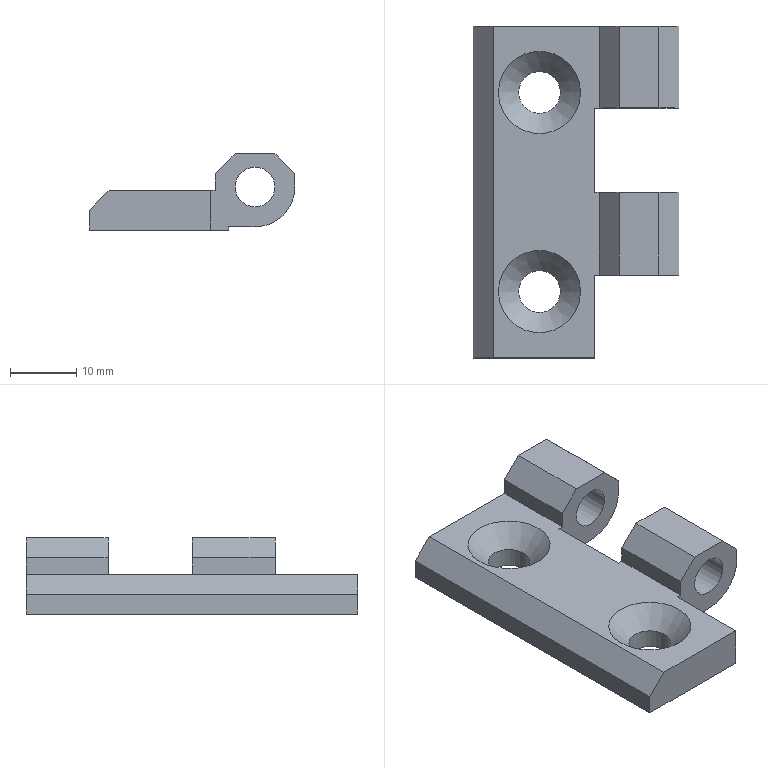Part | STEP file | C_HHSZ50_pr | 1 solid | 33 faces | box 31 x 50 x 11.5 mm | volume 6935 mm3 | plane 25 | cylinder 6 | cone 2 | commonest cylinder face diameters 6 x2 6.3 x2 12 x2
STEP:
#1=CARTESIAN_POINT('',(-11.85,15.,0.));
#2=VERTEX_POINT('',#1);
#3=CARTESIAN_POINT('',(-15.,15.,0.));
#4=DIRECTION('',(0.,0.,1.));
#5=DIRECTION('',(1.,0.,0.));
#6=AXIS2_PLACEMENT_3D('',#3,#4,#5);
#7=CIRCLE('',#6,3.15);
#8=EDGE_CURVE('',#2,#2,#7,.T.);
#9=ORIENTED_EDGE('',*,*,#8,.T.);
#10=EDGE_LOOP('',(#9));
#11=FACE_BOUND('',#10,.T.);
#12=CARTESIAN_POINT('',(-4.,12.65,0.));
#13=VERTEX_POINT('',#12);
#14=CARTESIAN_POINT('',(-6.7,12.65,0.));
#15=VERTEX_POINT('',#14);
#16=CARTESIAN_POINT('',(6.7,12.65,0.));
#17=DIRECTION('',(-1.,0.,0.));
#18=VECTOR('',#17,1000.);
#19=LINE('',#16,#18);
#20=EDGE_CURVE('',#13,#15,#19,.T.);
#21=ORIENTED_EDGE('',*,*,#20,.T.);
#22=CARTESIAN_POINT('',(-6.7,-0.05,0.));
#23=VERTEX_POINT('',#22);
#24=CARTESIAN_POINT('',(-6.7,12.65,0.));
#25=DIRECTION('',(0.,-1.,0.));
#26=VECTOR('',#25,1000.);
#27=LINE('',#24,#26);
#28=EDGE_CURVE('',#15,#23,#27,.T.);
#29=ORIENTED_EDGE('',*,*,#28,.T.);
#30=CARTESIAN_POINT('',(-4.,-0.05,0.));
#31=VERTEX_POINT('',#30);
#32=CARTESIAN_POINT('',(-6.7,-0.05,0.));
#33=DIRECTION('',(1.,0.,0.));
#34=VECTOR('',#33,1000.);
#35=LINE('',#32,#34);
#36=EDGE_CURVE('',#23,#31,#35,.T.);
#37=ORIENTED_EDGE('',*,*,#36,.T.);
#38=CARTESIAN_POINT('',(-4.,-12.55,0.));
#39=VERTEX_POINT('',#38);
#40=CARTESIAN_POINT('',(-4.,25.,0.));
#41=DIRECTION('',(0.,-1.,0.));
#42=VECTOR('',#41,1000.);
#43=LINE('',#40,#42);
#44=EDGE_CURVE('',#31,#39,#43,.T.);
#45=ORIENTED_EDGE('',*,*,#44,.T.);
#46=CARTESIAN_POINT('',(-6.7,-12.55,0.));
#47=VERTEX_POINT('',#46);
#48=CARTESIAN_POINT('',(6.7,-12.55,0.));
#49=DIRECTION('',(-1.,0.,0.));
#50=VECTOR('',#49,1000.);
#51=LINE('',#48,#50);
#52=EDGE_CURVE('',#39,#47,#51,.T.);
#53=ORIENTED_EDGE('',*,*,#52,.T.);
#54=CARTESIAN_POINT('',(-6.7,-25.,0.));
#55=VERTEX_POINT('',#54);
#56=CARTESIAN_POINT('',(-6.7,-12.55,0.));
#57=DIRECTION('',(0.,-1.,0.));
#58=VECTOR('',#57,1000.);
#59=LINE('',#56,#58);
#60=EDGE_CURVE('',#47,#55,#59,.T.);
#61=ORIENTED_EDGE('',*,*,#60,.T.);
#62=CARTESIAN_POINT('',(-25.,-25.,0.));
#63=VERTEX_POINT('',#62);
#64=CARTESIAN_POINT('',(-4.,-25.,0.));
#65=DIRECTION('',(-1.,0.,0.));
#66=VECTOR('',#65,1000.);
#67=LINE('',#64,#66);
#68=EDGE_CURVE('',#55,#63,#67,.T.);
#69=ORIENTED_EDGE('',*,*,#68,.T.);
#70=CARTESIAN_POINT('',(-25.,25.,0.));
#71=VERTEX_POINT('',#70);
#72=CARTESIAN_POINT('',(-25.,25.,0.));
#73=DIRECTION('',(0.,-1.,0.));
#74=VECTOR('',#73,1000.);
#75=LINE('',#72,#74);
#76=EDGE_CURVE('',#71,#63,#75,.T.);
#77=ORIENTED_EDGE('',*,*,#76,.F.);
#78=CARTESIAN_POINT('',(-4.,25.,0.));
#79=VERTEX_POINT('',#78);
#80=CARTESIAN_POINT('',(-4.,25.,0.));
#81=DIRECTION('',(-1.,0.,0.));
#82=VECTOR('',#81,1000.);
#83=LINE('',#80,#82);
#84=EDGE_CURVE('',#79,#71,#83,.T.);
#85=ORIENTED_EDGE('',*,*,#84,.F.);
#86=CARTESIAN_POINT('',(-4.,25.,0.));
#87=DIRECTION('',(0.,-1.,0.));
#88=VECTOR('',#87,1000.);
#89=LINE('',#86,#88);
#90=EDGE_CURVE('',#79,#13,#89,.T.);
#91=ORIENTED_EDGE('',*,*,#90,.T.);
#92=EDGE_LOOP('',(#21,#29,#37,#45,#53,#61,#69,#77,#85,#91));
#93=FACE_OUTER_BOUND('',#92,.T.);
#94=CARTESIAN_POINT('',(-11.85,-15.,0.));
#95=VERTEX_POINT('',#94);
#96=CARTESIAN_POINT('',(-15.,-15.,0.));
#97=DIRECTION('',(0.,0.,1.));
#98=DIRECTION('',(1.,0.,0.));
#99=AXIS2_PLACEMENT_3D('',#96,#97,#98);
#100=CIRCLE('',#99,3.15);
#101=EDGE_CURVE('',#95,#95,#100,.T.);
#102=ORIENTED_EDGE('',*,*,#101,.T.);
#103=EDGE_LOOP('',(#102));
#104=FACE_BOUND('',#103,.T.);
#105=CARTESIAN_POINT('',(-4.,25.,0.));
#106=DIRECTION('',(0.,0.,1.));
#107=DIRECTION('',(1.,0.,0.));
#108=AXIS2_PLACEMENT_3D('',#105,#106,#107);
#109=PLANE('',#108);
#110=ADVANCED_FACE('',(#11,#93,#104),#109,.F.);
#111=CARTESIAN_POINT('',(-8.8,15.,6.));
#112=VERTEX_POINT('',#111);
#113=CARTESIAN_POINT('',(-15.,15.,6.));
#114=DIRECTION('',(0.,0.,1.));
#115=DIRECTION('',(1.,0.,0.));
#116=AXIS2_PLACEMENT_3D('',#113,#114,#115);
#117=CIRCLE('',#116,6.2);
#118=EDGE_CURVE('',#112,#112,#117,.T.);
#119=ORIENTED_EDGE('',*,*,#118,.F.);
#120=EDGE_LOOP('',(#119));
#121=FACE_BOUND('',#120,.T.);
#122=CARTESIAN_POINT('',(-6.,12.65,6.));
#123=VERTEX_POINT('',#122);
#124=CARTESIAN_POINT('',(-6.7,12.65,6.));
#125=VERTEX_POINT('',#124);
#126=CARTESIAN_POINT('',(-22.,12.65,6.));
#127=DIRECTION('',(-1.,0.,0.));
#128=VECTOR('',#127,1000.);
#129=LINE('',#126,#128);
#130=EDGE_CURVE('',#123,#125,#129,.T.);
#131=ORIENTED_EDGE('',*,*,#130,.F.);
#132=CARTESIAN_POINT('',(-6.,25.,6.));
#133=VERTEX_POINT('',#132);
#134=CARTESIAN_POINT('',(-6.,25.,6.));
#135=DIRECTION('',(0.,-1.,0.));
#136=VECTOR('',#135,1000.);
#137=LINE('',#134,#136);
#138=EDGE_CURVE('',#133,#123,#137,.T.);
#139=ORIENTED_EDGE('',*,*,#138,.F.);
#140=CARTESIAN_POINT('',(-22.,25.,6.));
#141=VERTEX_POINT('',#140);
#142=CARTESIAN_POINT('',(-22.,25.,6.));
#143=DIRECTION('',(1.,0.,0.));
#144=VECTOR('',#143,1000.);
#145=LINE('',#142,#144);
#146=EDGE_CURVE('',#141,#133,#145,.T.);
#147=ORIENTED_EDGE('',*,*,#146,.F.);
#148=CARTESIAN_POINT('',(-22.,-25.,6.));
#149=VERTEX_POINT('',#148);
#150=CARTESIAN_POINT('',(-22.,25.,6.));
#151=DIRECTION('',(0.,-1.,0.));
#152=VECTOR('',#151,1000.);
#153=LINE('',#150,#152);
#154=EDGE_CURVE('',#141,#149,#153,.T.);
#155=ORIENTED_EDGE('',*,*,#154,.T.);
#156=CARTESIAN_POINT('',(-6.7,-25.,6.));
#157=VERTEX_POINT('',#156);
#158=CARTESIAN_POINT('',(-22.,-25.,6.));
#159=DIRECTION('',(1.,0.,0.));
#160=VECTOR('',#159,1000.);
#161=LINE('',#158,#160);
#162=EDGE_CURVE('',#149,#157,#161,.T.);
#163=ORIENTED_EDGE('',*,*,#162,.T.);
#164=CARTESIAN_POINT('',(-6.7,-12.55,6.));
#165=VERTEX_POINT('',#164);
#166=CARTESIAN_POINT('',(-6.7,25.,6.));
#167=DIRECTION('',(0.,-1.,0.));
#168=VECTOR('',#167,1000.);
#169=LINE('',#166,#168);
#170=EDGE_CURVE('',#165,#157,#169,.T.);
#171=ORIENTED_EDGE('',*,*,#170,.F.);
#172=CARTESIAN_POINT('',(-6.,-12.55,6.));
#173=VERTEX_POINT('',#172);
#174=CARTESIAN_POINT('',(-22.,-12.55,6.));
#175=DIRECTION('',(-1.,0.,0.));
#176=VECTOR('',#175,1000.);
#177=LINE('',#174,#176);
#178=EDGE_CURVE('',#173,#165,#177,.T.);
#179=ORIENTED_EDGE('',*,*,#178,.F.);
#180=CARTESIAN_POINT('',(-6.,-0.05,6.));
#181=VERTEX_POINT('',#180);
#182=CARTESIAN_POINT('',(-6.,25.,6.));
#183=DIRECTION('',(0.,-1.,0.));
#184=VECTOR('',#183,1000.);
#185=LINE('',#182,#184);
#186=EDGE_CURVE('',#181,#173,#185,.T.);
#187=ORIENTED_EDGE('',*,*,#186,.F.);
#188=CARTESIAN_POINT('',(-6.7,-0.05,6.));
#189=VERTEX_POINT('',#188);
#190=CARTESIAN_POINT('',(-22.,-0.05,6.));
#191=DIRECTION('',(1.,0.,0.));
#192=VECTOR('',#191,1000.);
#193=LINE('',#190,#192);
#194=EDGE_CURVE('',#189,#181,#193,.T.);
#195=ORIENTED_EDGE('',*,*,#194,.F.);
#196=CARTESIAN_POINT('',(-6.7,25.,6.));
#197=DIRECTION('',(0.,-1.,0.));
#198=VECTOR('',#197,1000.);
#199=LINE('',#196,#198);
#200=EDGE_CURVE('',#125,#189,#199,.T.);
#201=ORIENTED_EDGE('',*,*,#200,.F.);
#202=EDGE_LOOP('',(#131,#139,#147,#155,#163,#171,#179,#187,#195,#201));
#203=FACE_OUTER_BOUND('',#202,.T.);
#204=CARTESIAN_POINT('',(-8.8,-15.,6.));
#205=VERTEX_POINT('',#204);
#206=CARTESIAN_POINT('',(-15.,-15.,6.));
#207=DIRECTION('',(0.,0.,1.));
#208=DIRECTION('',(1.,0.,0.));
#209=AXIS2_PLACEMENT_3D('',#206,#207,#208);
#210=CIRCLE('',#209,6.2);
#211=EDGE_CURVE('',#205,#205,#210,.T.);
#212=ORIENTED_EDGE('',*,*,#211,.F.);
#213=EDGE_LOOP('',(#212));
#214=FACE_BOUND('',#213,.T.);
#215=CARTESIAN_POINT('',(-22.,25.,6.));
#216=DIRECTION('',(0.,0.,-1.));
#217=DIRECTION('',(-1.,0.,0.));
#218=AXIS2_PLACEMENT_3D('',#215,#216,#217);
#219=PLANE('',#218);
#220=ADVANCED_FACE('',(#121,#203,#214),#219,.F.);
#221=CARTESIAN_POINT('',(-6.,12.65,8.5));
#222=VERTEX_POINT('',#221);
#223=CARTESIAN_POINT('',(-6.,12.65,6.));
#224=DIRECTION('',(0.,0.,-1.));
#225=VECTOR('',#224,1000.);
#226=LINE('',#223,#225);
#227=EDGE_CURVE('',#222,#123,#226,.T.);
#228=ORIENTED_EDGE('',*,*,#227,.F.);
#229=CARTESIAN_POINT('',(-6.,25.,8.5));
#230=VERTEX_POINT('',#229);
#231=CARTESIAN_POINT('',(-6.,25.,8.5));
#232=DIRECTION('',(0.,-1.,0.));
#233=VECTOR('',#232,1000.);
#234=LINE('',#231,#233);
#235=EDGE_CURVE('',#230,#222,#234,.T.);
#236=ORIENTED_EDGE('',*,*,#235,.F.);
#237=CARTESIAN_POINT('',(-6.,25.,6.));
#238=DIRECTION('',(0.,0.,1.));
#239=VECTOR('',#238,1000.);
#240=LINE('',#237,#239);
#241=EDGE_CURVE('',#133,#230,#240,.T.);
#242=ORIENTED_EDGE('',*,*,#241,.F.);
#243=ORIENTED_EDGE('',*,*,#138,.T.);
#244=EDGE_LOOP('',(#228,#236,#242,#243));
#245=FACE_OUTER_BOUND('',#244,.T.);
#246=CARTESIAN_POINT('',(-6.,25.,6.));
#247=DIRECTION('',(1.,0.,0.));
#248=DIRECTION('',(0.,0.,-1.));
#249=AXIS2_PLACEMENT_3D('',#246,#247,#248);
#250=PLANE('',#249);
#251=ADVANCED_FACE('',(#245),#250,.F.);
#252=CARTESIAN_POINT('',(-6.,-0.05,8.5));
#253=VERTEX_POINT('',#252);
#254=CARTESIAN_POINT('',(-6.,-0.05,6.));
#255=DIRECTION('',(0.,0.,1.));
#256=VECTOR('',#255,1000.);
#257=LINE('',#254,#256);
#258=EDGE_CURVE('',#181,#253,#257,.T.);
#259=ORIENTED_EDGE('',*,*,#258,.F.);
#260=ORIENTED_EDGE('',*,*,#186,.T.);
#261=CARTESIAN_POINT('',(-6.,-12.55,8.5));
#262=VERTEX_POINT('',#261);
#263=CARTESIAN_POINT('',(-6.,-12.55,6.));
#264=DIRECTION('',(0.,0.,-1.));
#265=VECTOR('',#264,1000.);
#266=LINE('',#263,#265);
#267=EDGE_CURVE('',#262,#173,#266,.T.);
#268=ORIENTED_EDGE('',*,*,#267,.F.);
#269=CARTESIAN_POINT('',(-6.,25.,8.5));
#270=DIRECTION('',(0.,-1.,0.));
#271=VECTOR('',#270,1000.);
#272=LINE('',#269,#271);
#273=EDGE_CURVE('',#253,#262,#272,.T.);
#274=ORIENTED_EDGE('',*,*,#273,.F.);
#275=EDGE_LOOP('',(#259,#260,#268,#274));
#276=FACE_OUTER_BOUND('',#275,.T.);
#277=CARTESIAN_POINT('',(-6.,25.,6.));
#278=DIRECTION('',(1.,0.,0.));
#279=DIRECTION('',(0.,0.,-1.));
#280=AXIS2_PLACEMENT_3D('',#277,#278,#279);
#281=PLANE('',#280);
#282=ADVANCED_FACE('',(#276),#281,.F.);
#283=CARTESIAN_POINT('',(-3.,12.65,11.5));
#284=VERTEX_POINT('',#283);
#285=CARTESIAN_POINT('',(-6.,12.65,8.5));
#286=DIRECTION('',(-0.7071,0.,-0.7071));
#287=VECTOR('',#286,1000.);
#288=LINE('',#285,#287);
#289=EDGE_CURVE('',#284,#222,#288,.T.);
#290=ORIENTED_EDGE('',*,*,#289,.F.);
#291=CARTESIAN_POINT('',(-3.,25.,11.5));
#292=VERTEX_POINT('',#291);
#293=CARTESIAN_POINT('',(-3.,25.,11.5));
#294=DIRECTION('',(0.,-1.,0.));
#295=VECTOR('',#294,1000.);
#296=LINE('',#293,#295);
#297=EDGE_CURVE('',#292,#284,#296,.T.);
#298=ORIENTED_EDGE('',*,*,#297,.F.);
#299=CARTESIAN_POINT('',(-6.,25.,8.5));
#300=DIRECTION('',(0.7071,0.,0.7071));
#301=VECTOR('',#300,1000.);
#302=LINE('',#299,#301);
#303=EDGE_CURVE('',#230,#292,#302,.T.);
#304=ORIENTED_EDGE('',*,*,#303,.F.);
#305=ORIENTED_EDGE('',*,*,#235,.T.);
#306=EDGE_LOOP('',(#290,#298,#304,#305));
#307=FACE_OUTER_BOUND('',#306,.T.);
#308=CARTESIAN_POINT('',(-6.,25.,8.5));
#309=DIRECTION('',(0.7071,0.,-0.7071));
#310=DIRECTION('',(-0.7071,0.,-0.7071));
#311=AXIS2_PLACEMENT_3D('',#308,#309,#310);
#312=PLANE('',#311);
#313=ADVANCED_FACE('',(#307),#312,.F.);
#314=CARTESIAN_POINT('',(-3.,-0.05,11.5));
#315=VERTEX_POINT('',#314);
#316=CARTESIAN_POINT('',(-6.,-0.05,8.5));
#317=DIRECTION('',(0.7071,0.,0.7071));
#318=VECTOR('',#317,1000.);
#319=LINE('',#316,#318);
#320=EDGE_CURVE('',#253,#315,#319,.T.);
#321=ORIENTED_EDGE('',*,*,#320,.F.);
#322=ORIENTED_EDGE('',*,*,#273,.T.);
#323=CARTESIAN_POINT('',(-3.,-12.55,11.5));
#324=VERTEX_POINT('',#323);
#325=CARTESIAN_POINT('',(-6.,-12.55,8.5));
#326=DIRECTION('',(-0.7071,0.,-0.7071));
#327=VECTOR('',#326,1000.);
#328=LINE('',#325,#327);
#329=EDGE_CURVE('',#324,#262,#328,.T.);
#330=ORIENTED_EDGE('',*,*,#329,.F.);
#331=CARTESIAN_POINT('',(-3.,25.,11.5));
#332=DIRECTION('',(0.,-1.,0.));
#333=VECTOR('',#332,1000.);
#334=LINE('',#331,#333);
#335=EDGE_CURVE('',#315,#324,#334,.T.);
#336=ORIENTED_EDGE('',*,*,#335,.F.);
#337=EDGE_LOOP('',(#321,#322,#330,#336));
#338=FACE_OUTER_BOUND('',#337,.T.);
#339=CARTESIAN_POINT('',(-6.,25.,8.5));
#340=DIRECTION('',(0.7071,0.,-0.7071));
#341=DIRECTION('',(-0.7071,0.,-0.7071));
#342=AXIS2_PLACEMENT_3D('',#339,#340,#341);
#343=PLANE('',#342);
#344=ADVANCED_FACE('',(#338),#343,.F.);
#345=CARTESIAN_POINT('',(3.,12.65,11.5));
#346=VERTEX_POINT('',#345);
#347=CARTESIAN_POINT('',(-3.,12.65,11.5));
#348=DIRECTION('',(-1.,0.,0.));
#349=VECTOR('',#348,1000.);
#350=LINE('',#347,#349);
#351=EDGE_CURVE('',#346,#284,#350,.T.);
#352=ORIENTED_EDGE('',*,*,#351,.F.);
#353=CARTESIAN_POINT('',(3.,25.,11.5));
#354=VERTEX_POINT('',#353);
#355=CARTESIAN_POINT('',(3.,25.,11.5));
#356=DIRECTION('',(0.,-1.,0.));
#357=VECTOR('',#356,1000.);
#358=LINE('',#355,#357);
#359=EDGE_CURVE('',#354,#346,#358,.T.);
#360=ORIENTED_EDGE('',*,*,#359,.F.);
#361=CARTESIAN_POINT('',(-3.,25.,11.5));
#362=DIRECTION('',(1.,0.,0.));
#363=VECTOR('',#362,1000.);
#364=LINE('',#361,#363);
#365=EDGE_CURVE('',#292,#354,#364,.T.);
#366=ORIENTED_EDGE('',*,*,#365,.F.);
#367=ORIENTED_EDGE('',*,*,#297,.T.);
#368=EDGE_LOOP('',(#352,#360,#366,#367));
#369=FACE_OUTER_BOUND('',#368,.T.);
#370=CARTESIAN_POINT('',(-3.,25.,11.5));
#371=DIRECTION('',(0.,0.,-1.));
#372=DIRECTION('',(-1.,0.,0.));
#373=AXIS2_PLACEMENT_3D('',#370,#371,#372);
#374=PLANE('',#373);
#375=ADVANCED_FACE('',(#369),#374,.F.);
#376=CARTESIAN_POINT('',(3.,-0.05,11.5));
#377=VERTEX_POINT('',#376);
#378=CARTESIAN_POINT('',(-3.,-0.05,11.5));
#379=DIRECTION('',(1.,0.,0.));
#380=VECTOR('',#379,1000.);
#381=LINE('',#378,#380);
#382=EDGE_CURVE('',#315,#377,#381,.T.);
#383=ORIENTED_EDGE('',*,*,#382,.F.);
#384=ORIENTED_EDGE('',*,*,#335,.T.);
#385=CARTESIAN_POINT('',(3.,-12.55,11.5));
#386=VERTEX_POINT('',#385);
#387=CARTESIAN_POINT('',(-3.,-12.55,11.5));
#388=DIRECTION('',(-1.,0.,0.));
#389=VECTOR('',#388,1000.);
#390=LINE('',#387,#389);
#391=EDGE_CURVE('',#386,#324,#390,.T.);
#392=ORIENTED_EDGE('',*,*,#391,.F.);
#393=CARTESIAN_POINT('',(3.,25.,11.5));
#394=DIRECTION('',(0.,-1.,0.));
#395=VECTOR('',#394,1000.);
#396=LINE('',#393,#395);
#397=EDGE_CURVE('',#377,#386,#396,.T.);
#398=ORIENTED_EDGE('',*,*,#397,.F.);
#399=EDGE_LOOP('',(#383,#384,#392,#398));
#400=FACE_OUTER_BOUND('',#399,.T.);
#401=CARTESIAN_POINT('',(-3.,25.,11.5));
#402=DIRECTION('',(0.,0.,-1.));
#403=DIRECTION('',(-1.,0.,0.));
#404=AXIS2_PLACEMENT_3D('',#401,#402,#403);
#405=PLANE('',#404);
#406=ADVANCED_FACE('',(#400),#405,.F.);
#407=CARTESIAN_POINT('',(6.,12.65,8.5));
#408=VERTEX_POINT('',#407);
#409=CARTESIAN_POINT('',(3.,12.65,11.5));
#410=DIRECTION('',(-0.7071,0.,0.7071));
#411=VECTOR('',#410,1000.);
#412=LINE('',#409,#411);
#413=EDGE_CURVE('',#408,#346,#412,.T.);
#414=ORIENTED_EDGE('',*,*,#413,.F.);
#415=CARTESIAN_POINT('',(6.,25.,8.5));
#416=VERTEX_POINT('',#415);
#417=CARTESIAN_POINT('',(6.,25.,8.5));
#418=DIRECTION('',(0.,-1.,0.));
#419=VECTOR('',#418,1000.);
#420=LINE('',#417,#419);
#421=EDGE_CURVE('',#416,#408,#420,.T.);
#422=ORIENTED_EDGE('',*,*,#421,.F.);
#423=CARTESIAN_POINT('',(3.,25.,11.5));
#424=DIRECTION('',(0.7071,0.,-0.7071));
#425=VECTOR('',#424,1000.);
#426=LINE('',#423,#425);
#427=EDGE_CURVE('',#354,#416,#426,.T.);
#428=ORIENTED_EDGE('',*,*,#427,.F.);
#429=ORIENTED_EDGE('',*,*,#359,.T.);
#430=EDGE_LOOP('',(#414,#422,#428,#429));
#431=FACE_OUTER_BOUND('',#430,.T.);
#432=CARTESIAN_POINT('',(3.,25.,11.5));
#433=DIRECTION('',(-0.7071,0.,-0.7071));
#434=DIRECTION('',(-0.7071,0.,0.7071));
#435=AXIS2_PLACEMENT_3D('',#432,#433,#434);
#436=PLANE('',#435);
#437=ADVANCED_FACE('',(#431),#436,.F.);
#438=CARTESIAN_POINT('',(6.,-0.05,8.5));
#439=VERTEX_POINT('',#438);
#440=CARTESIAN_POINT('',(3.,-0.05,11.5));
#441=DIRECTION('',(0.7071,0.,-0.7071));
#442=VECTOR('',#441,1000.);
#443=LINE('',#440,#442);
#444=EDGE_CURVE('',#377,#439,#443,.T.);
#445=ORIENTED_EDGE('',*,*,#444,.F.);
#446=ORIENTED_EDGE('',*,*,#397,.T.);
#447=CARTESIAN_POINT('',(6.,-12.55,8.5));
#448=VERTEX_POINT('',#447);
#449=CARTESIAN_POINT('',(3.,-12.55,11.5));
#450=DIRECTION('',(-0.7071,0.,0.7071));
#451=VECTOR('',#450,1000.);
#452=LINE('',#449,#451);
#453=EDGE_CURVE('',#448,#386,#452,.T.);
#454=ORIENTED_EDGE('',*,*,#453,.F.);
#455=CARTESIAN_POINT('',(6.,25.,8.5));
#456=DIRECTION('',(0.,-1.,0.));
#457=VECTOR('',#456,1000.);
#458=LINE('',#455,#457);
#459=EDGE_CURVE('',#439,#448,#458,.T.);
#460=ORIENTED_EDGE('',*,*,#459,.F.);
#461=EDGE_LOOP('',(#445,#446,#454,#460));
#462=FACE_OUTER_BOUND('',#461,.T.);
#463=CARTESIAN_POINT('',(3.,25.,11.5));
#464=DIRECTION('',(-0.7071,0.,-0.7071));
#465=DIRECTION('',(-0.7071,0.,0.7071));
#466=AXIS2_PLACEMENT_3D('',#463,#464,#465);
#467=PLANE('',#466);
#468=ADVANCED_FACE('',(#462),#467,.F.);
#469=CARTESIAN_POINT('',(6.,12.65,6.5));
#470=VERTEX_POINT('',#469);
#471=CARTESIAN_POINT('',(6.,12.65,8.5));
#472=DIRECTION('',(0.,0.,1.));
#473=VECTOR('',#472,1000.);
#474=LINE('',#471,#473);
#475=EDGE_CURVE('',#470,#408,#474,.T.);
#476=ORIENTED_EDGE('',*,*,#475,.F.);
#477=CARTESIAN_POINT('',(6.,25.,6.5));
#478=VERTEX_POINT('',#477);
#479=CARTESIAN_POINT('',(6.,25.,6.5));
#480=DIRECTION('',(0.,-1.,0.));
#481=VECTOR('',#480,1000.);
#482=LINE('',#479,#481);
#483=EDGE_CURVE('',#478,#470,#482,.T.);
#484=ORIENTED_EDGE('',*,*,#483,.F.);
#485=CARTESIAN_POINT('',(6.,25.,8.5));
#486=DIRECTION('',(0.,0.,-1.));
#487=VECTOR('',#486,1000.);
#488=LINE('',#485,#487);
#489=EDGE_CURVE('',#416,#478,#488,.T.);
#490=ORIENTED_EDGE('',*,*,#489,.F.);
#491=ORIENTED_EDGE('',*,*,#421,.T.);
#492=EDGE_LOOP('',(#476,#484,#490,#491));
#493=FACE_OUTER_BOUND('',#492,.T.);
#494=CARTESIAN_POINT('',(6.,25.,8.5));
#495=DIRECTION('',(-1.,0.,0.));
#496=DIRECTION('',(0.,0.,1.));
#497=AXIS2_PLACEMENT_3D('',#494,#495,#496);
#498=PLANE('',#497);
#499=ADVANCED_FACE('',(#493),#498,.F.);
#500=CARTESIAN_POINT('',(6.,-0.05,6.5));
#501=VERTEX_POINT('',#500);
#502=CARTESIAN_POINT('',(6.,-0.05,8.5));
#503=DIRECTION('',(0.,0.,-1.));
#504=VECTOR('',#503,1000.);
#505=LINE('',#502,#504);
#506=EDGE_CURVE('',#439,#501,#505,.T.);
#507=ORIENTED_EDGE('',*,*,#506,.F.);
#508=ORIENTED_EDGE('',*,*,#459,.T.);
#509=CARTESIAN_POINT('',(6.,-12.55,6.5));
#510=VERTEX_POINT('',#509);
#511=CARTESIAN_POINT('',(6.,-12.55,8.5));
#512=DIRECTION('',(0.,0.,1.));
#513=VECTOR('',#512,1000.);
#514=LINE('',#511,#513);
#515=EDGE_CURVE('',#510,#448,#514,.T.);
#516=ORIENTED_EDGE('',*,*,#515,.F.);
#517=CARTESIAN_POINT('',(6.,25.,6.5));
#518=DIRECTION('',(0.,-1.,0.));
#519=VECTOR('',#518,1000.);
#520=LINE('',#517,#519);
#521=EDGE_CURVE('',#501,#510,#520,.T.);
#522=ORIENTED_EDGE('',*,*,#521,.F.);
#523=EDGE_LOOP('',(#507,#508,#516,#522));
#524=FACE_OUTER_BOUND('',#523,.T.);
#525=CARTESIAN_POINT('',(6.,25.,8.5));
#526=DIRECTION('',(-1.,0.,0.));
#527=DIRECTION('',(0.,0.,1.));
#528=AXIS2_PLACEMENT_3D('',#525,#526,#527);
#529=PLANE('',#528);
#530=ADVANCED_FACE('',(#524),#529,.F.);
#531=CARTESIAN_POINT('',(0.,12.65,0.5));
#532=VERTEX_POINT('',#531);
#533=CARTESIAN_POINT('',(0.,12.65,6.5));
#534=DIRECTION('',(0.,-1.,0.));
#535=DIRECTION('',(0.,0.,-1.));
#536=AXIS2_PLACEMENT_3D('',#533,#534,#535);
#537=CIRCLE('',#536,6.);
#538=EDGE_CURVE('',#532,#470,#537,.T.);
#539=ORIENTED_EDGE('',*,*,#538,.F.);
#540=CARTESIAN_POINT('',(0.,25.,0.5));
#541=VERTEX_POINT('',#540);
#542=CARTESIAN_POINT('',(0.,25.,0.5));
#543=DIRECTION('',(0.,-1.,0.));
#544=VECTOR('',#543,1000.);
#545=LINE('',#542,#544);
#546=EDGE_CURVE('',#541,#532,#545,.T.);
#547=ORIENTED_EDGE('',*,*,#546,.F.);
#548=CARTESIAN_POINT('',(0.,25.,6.5));
#549=DIRECTION('',(0.,1.,0.));
#550=DIRECTION('',(0.,0.,1.));
#551=AXIS2_PLACEMENT_3D('',#548,#549,#550);
#552=CIRCLE('',#551,6.);
#553=EDGE_CURVE('',#478,#541,#552,.T.);
#554=ORIENTED_EDGE('',*,*,#553,.F.);
#555=ORIENTED_EDGE('',*,*,#483,.T.);
#556=EDGE_LOOP('',(#539,#547,#554,#555));
#557=FACE_OUTER_BOUND('',#556,.T.);
#558=CARTESIAN_POINT('',(0.,25.,6.5));
#559=DIRECTION('',(0.,-1.,0.));
#560=DIRECTION('',(0.,0.,-1.));
#561=AXIS2_PLACEMENT_3D('',#558,#559,#560);
#562=CYLINDRICAL_SURFACE('',#561,6.);
#563=ADVANCED_FACE('',(#557),#562,.T.);
#564=CARTESIAN_POINT('',(0.,-0.05,0.5));
#565=VERTEX_POINT('',#564);
#566=CARTESIAN_POINT('',(0.,-0.05,6.5));
#567=DIRECTION('',(0.,1.,0.));
#568=DIRECTION('',(0.,0.,1.));
#569=AXIS2_PLACEMENT_3D('',#566,#567,#568);
#570=CIRCLE('',#569,6.);
#571=EDGE_CURVE('',#501,#565,#570,.T.);
#572=ORIENTED_EDGE('',*,*,#571,.F.);
#573=ORIENTED_EDGE('',*,*,#521,.T.);
#574=CARTESIAN_POINT('',(0.,-12.55,0.5));
#575=VERTEX_POINT('',#574);
#576=CARTESIAN_POINT('',(0.,-12.55,6.5));
#577=DIRECTION('',(0.,-1.,0.));
#578=DIRECTION('',(0.,0.,-1.));
#579=AXIS2_PLACEMENT_3D('',#576,#577,#578);
#580=CIRCLE('',#579,6.);
#581=EDGE_CURVE('',#575,#510,#580,.T.);
#582=ORIENTED_EDGE('',*,*,#581,.F.);
#583=CARTESIAN_POINT('',(0.,25.,0.5));
#584=DIRECTION('',(0.,-1.,0.));
#585=VECTOR('',#584,1000.);
#586=LINE('',#583,#585);
#587=EDGE_CURVE('',#565,#575,#586,.T.);
#588=ORIENTED_EDGE('',*,*,#587,.F.);
#589=EDGE_LOOP('',(#572,#573,#582,#588));
#590=FACE_OUTER_BOUND('',#589,.T.);
#591=CARTESIAN_POINT('',(0.,25.,6.5));
#592=DIRECTION('',(0.,-1.,0.));
#593=DIRECTION('',(0.,0.,-1.));
#594=AXIS2_PLACEMENT_3D('',#591,#592,#593);
#595=CYLINDRICAL_SURFACE('',#594,6.);
#596=ADVANCED_FACE('',(#590),#595,.T.);
#597=CARTESIAN_POINT('',(-4.,12.65,0.5));
#598=VERTEX_POINT('',#597);
#599=CARTESIAN_POINT('',(0.,12.65,0.5));
#600=DIRECTION('',(1.,0.,0.));
#601=VECTOR('',#600,1000.);
#602=LINE('',#599,#601);
#603=EDGE_CURVE('',#598,#532,#602,.T.);
#604=ORIENTED_EDGE('',*,*,#603,.F.);
#605=CARTESIAN_POINT('',(-4.,25.,0.5));
#606=VERTEX_POINT('',#605);
#607=CARTESIAN_POINT('',(-4.,25.,0.5));
#608=DIRECTION('',(0.,-1.,0.));
#609=VECTOR('',#608,1000.);
#610=LINE('',#607,#609);
#611=EDGE_CURVE('',#606,#598,#610,.T.);
#612=ORIENTED_EDGE('',*,*,#611,.F.);
#613=CARTESIAN_POINT('',(0.,25.,0.5));
#614=DIRECTION('',(-1.,0.,0.));
#615=VECTOR('',#614,1000.);
#616=LINE('',#613,#615);
#617=EDGE_CURVE('',#541,#606,#616,.T.);
#618=ORIENTED_EDGE('',*,*,#617,.F.);
#619=ORIENTED_EDGE('',*,*,#546,.T.);
#620=EDGE_LOOP('',(#604,#612,#618,#619));
#621=FACE_OUTER_BOUND('',#620,.T.);
#622=CARTESIAN_POINT('',(0.,25.,0.5));
#623=DIRECTION('',(0.,0.,1.));
#624=DIRECTION('',(1.,0.,0.));
#625=AXIS2_PLACEMENT_3D('',#622,#623,#624);
#626=PLANE('',#625);
#627=ADVANCED_FACE('',(#621),#626,.F.);
#628=CARTESIAN_POINT('',(-4.,-0.05,0.5));
#629=VERTEX_POINT('',#628);
#630=CARTESIAN_POINT('',(0.,-0.05,0.5));
#631=DIRECTION('',(-1.,0.,0.));
#632=VECTOR('',#631,1000.);
#633=LINE('',#630,#632);
#634=EDGE_CURVE('',#565,#629,#633,.T.);
#635=ORIENTED_EDGE('',*,*,#634,.F.);
#636=ORIENTED_EDGE('',*,*,#587,.T.);
#637=CARTESIAN_POINT('',(-4.,-12.55,0.5));
#638=VERTEX_POINT('',#637);
#639=CARTESIAN_POINT('',(0.,-12.55,0.5));
#640=DIRECTION('',(1.,0.,0.));
#641=VECTOR('',#640,1000.);
#642=LINE('',#639,#641);
#643=EDGE_CURVE('',#638,#575,#642,.T.);
#644=ORIENTED_EDGE('',*,*,#643,.F.);
#645=CARTESIAN_POINT('',(-4.,25.,0.5));
#646=DIRECTION('',(0.,-1.,0.));
#647=VECTOR('',#646,1000.);
#648=LINE('',#645,#647);
#649=EDGE_CURVE('',#629,#638,#648,.T.);
#650=ORIENTED_EDGE('',*,*,#649,.F.);
#651=EDGE_LOOP('',(#635,#636,#644,#650));
#652=FACE_OUTER_BOUND('',#651,.T.);
#653=CARTESIAN_POINT('',(0.,25.,0.5));
#654=DIRECTION('',(0.,0.,1.));
#655=DIRECTION('',(1.,0.,0.));
#656=AXIS2_PLACEMENT_3D('',#653,#654,#655);
#657=PLANE('',#656);
#658=ADVANCED_FACE('',(#652),#657,.F.);
#659=CARTESIAN_POINT('',(-4.,12.65,0.5));
#660=DIRECTION('',(0.,0.,1.));
#661=VECTOR('',#660,1000.);
#662=LINE('',#659,#661);
#663=EDGE_CURVE('',#13,#598,#662,.T.);
#664=ORIENTED_EDGE('',*,*,#663,.F.);
#665=ORIENTED_EDGE('',*,*,#90,.F.);
#666=CARTESIAN_POINT('',(-4.,25.,0.5));
#667=DIRECTION('',(0.,0.,-1.));
#668=VECTOR('',#667,1000.);
#669=LINE('',#666,#668);
#670=EDGE_CURVE('',#606,#79,#669,.T.);
#671=ORIENTED_EDGE('',*,*,#670,.F.);
#672=ORIENTED_EDGE('',*,*,#611,.T.);
#673=EDGE_LOOP('',(#664,#665,#671,#672));
#674=FACE_OUTER_BOUND('',#673,.T.);
#675=CARTESIAN_POINT('',(-4.,25.,0.5));
#676=DIRECTION('',(-1.,0.,0.));
#677=DIRECTION('',(0.,0.,1.));
#678=AXIS2_PLACEMENT_3D('',#675,#676,#677);
#679=PLANE('',#678);
#680=ADVANCED_FACE('',(#674),#679,.F.);
#681=CARTESIAN_POINT('',(-4.,-0.05,0.5));
#682=DIRECTION('',(0.,0.,-1.));
#683=VECTOR('',#682,1000.);
#684=LINE('',#681,#683);
#685=EDGE_CURVE('',#629,#31,#684,.T.);
#686=ORIENTED_EDGE('',*,*,#685,.F.);
#687=ORIENTED_EDGE('',*,*,#649,.T.);
#688=CARTESIAN_POINT('',(-4.,-12.55,0.5));
#689=DIRECTION('',(0.,0.,1.));
#690=VECTOR('',#689,1000.);
#691=LINE('',#688,#690);
#692=EDGE_CURVE('',#39,#638,#691,.T.);
#693=ORIENTED_EDGE('',*,*,#692,.F.);
#694=ORIENTED_EDGE('',*,*,#44,.F.);
#695=EDGE_LOOP('',(#686,#687,#693,#694));
#696=FACE_OUTER_BOUND('',#695,.T.);
#697=CARTESIAN_POINT('',(-4.,25.,0.5));
#698=DIRECTION('',(-1.,0.,0.));
#699=DIRECTION('',(0.,0.,1.));
#700=AXIS2_PLACEMENT_3D('',#697,#698,#699);
#701=PLANE('',#700);
#702=ADVANCED_FACE('',(#696),#701,.F.);
#703=CARTESIAN_POINT('',(0.,25.,9.5));
#704=VERTEX_POINT('',#703);
#705=CARTESIAN_POINT('',(0.,25.,6.5));
#706=DIRECTION('',(0.,1.,0.));
#707=DIRECTION('',(0.,0.,1.));
#708=AXIS2_PLACEMENT_3D('',#705,#706,#707);
#709=CIRCLE('',#708,3.);
#710=EDGE_CURVE('',#704,#704,#709,.T.);
#711=ORIENTED_EDGE('',*,*,#710,.T.);
#712=EDGE_LOOP('',(#711));
#713=FACE_OUTER_BOUND('',#712,.T.);
#714=CARTESIAN_POINT('',(0.,12.65,3.5));
#715=VERTEX_POINT('',#714);
#716=CARTESIAN_POINT('',(0.,12.65,6.5));
#717=DIRECTION('',(0.,-1.,0.));
#718=DIRECTION('',(0.,0.,-1.));
#719=AXIS2_PLACEMENT_3D('',#716,#717,#718);
#720=CIRCLE('',#719,3.);
#721=EDGE_CURVE('',#715,#715,#720,.T.);
#722=ORIENTED_EDGE('',*,*,#721,.T.);
#723=EDGE_LOOP('',(#722));
#724=FACE_OUTER_BOUND('',#723,.T.);
#725=CARTESIAN_POINT('',(0.,-25.,6.5));
#726=DIRECTION('',(0.,1.,0.));
#727=DIRECTION('',(0.,0.,1.));
#728=AXIS2_PLACEMENT_3D('',#725,#726,#727);
#729=CYLINDRICAL_SURFACE('',#728,3.);
#730=ADVANCED_FACE('',(#713,#724),#729,.F.);
#731=CARTESIAN_POINT('',(0.,-12.55,3.5));
#732=VERTEX_POINT('',#731);
#733=CARTESIAN_POINT('',(0.,-12.55,6.5));
#734=DIRECTION('',(0.,-1.,0.));
#735=DIRECTION('',(0.,0.,-1.));
#736=AXIS2_PLACEMENT_3D('',#733,#734,#735);
#737=CIRCLE('',#736,3.);
#738=EDGE_CURVE('',#732,#732,#737,.T.);
#739=ORIENTED_EDGE('',*,*,#738,.T.);
#740=EDGE_LOOP('',(#739));
#741=FACE_OUTER_BOUND('',#740,.T.);
#742=CARTESIAN_POINT('',(0.,-0.05,9.5));
#743=VERTEX_POINT('',#742);
#744=CARTESIAN_POINT('',(0.,-0.05,6.5));
#745=DIRECTION('',(0.,1.,0.));
#746=DIRECTION('',(0.,0.,1.));
#747=AXIS2_PLACEMENT_3D('',#744,#745,#746);
#748=CIRCLE('',#747,3.);
#749=EDGE_CURVE('',#743,#743,#748,.T.);
#750=ORIENTED_EDGE('',*,*,#749,.T.);
#751=EDGE_LOOP('',(#750));
#752=FACE_OUTER_BOUND('',#751,.T.);
#753=CARTESIAN_POINT('',(0.,-25.,6.5));
#754=DIRECTION('',(0.,1.,0.));
#755=DIRECTION('',(0.,0.,1.));
#756=AXIS2_PLACEMENT_3D('',#753,#754,#755);
#757=CYLINDRICAL_SURFACE('',#756,3.);
#758=ADVANCED_FACE('',(#741,#752),#757,.F.);
#759=CARTESIAN_POINT('',(-6.7,-25.,12.));
#760=DIRECTION('',(0.,0.,-1.));
#761=VECTOR('',#760,1000.);
#762=LINE('',#759,#761);
#763=EDGE_CURVE('',#157,#55,#762,.T.);
#764=ORIENTED_EDGE('',*,*,#763,.F.);
#765=ORIENTED_EDGE('',*,*,#162,.F.);
#766=CARTESIAN_POINT('',(-25.,-25.,3.));
#767=VERTEX_POINT('',#766);
#768=CARTESIAN_POINT('',(-25.,-25.,3.));
#769=DIRECTION('',(0.7071,0.,0.7071));
#770=VECTOR('',#769,1000.);
#771=LINE('',#768,#770);
#772=EDGE_CURVE('',#767,#149,#771,.T.);
#773=ORIENTED_EDGE('',*,*,#772,.F.);
#774=CARTESIAN_POINT('',(-25.,-25.,0.));
#775=DIRECTION('',(0.,0.,1.));
#776=VECTOR('',#775,1000.);
#777=LINE('',#774,#776);
#778=EDGE_CURVE('',#63,#767,#777,.T.);
#779=ORIENTED_EDGE('',*,*,#778,.F.);
#780=ORIENTED_EDGE('',*,*,#68,.F.);
#781=EDGE_LOOP('',(#764,#765,#773,#779,#780));
#782=FACE_OUTER_BOUND('',#781,.T.);
#783=CARTESIAN_POINT('',(0.,-25.,6.5));
#784=DIRECTION('',(0.,1.,0.));
#785=DIRECTION('',(0.,0.,1.));
#786=AXIS2_PLACEMENT_3D('',#783,#784,#785);
#787=PLANE('',#786);
#788=ADVANCED_FACE('',(#782),#787,.F.);
#789=ORIENTED_EDGE('',*,*,#84,.T.);
#790=CARTESIAN_POINT('',(-25.,25.,3.));
#791=VERTEX_POINT('',#790);
#792=CARTESIAN_POINT('',(-25.,25.,0.));
#793=DIRECTION('',(0.,0.,1.));
#794=VECTOR('',#793,1000.);
#795=LINE('',#792,#794);
#796=EDGE_CURVE('',#71,#791,#795,.T.);
#797=ORIENTED_EDGE('',*,*,#796,.T.);
#798=CARTESIAN_POINT('',(-25.,25.,3.));
#799=DIRECTION('',(0.7071,0.,0.7071));
#800=VECTOR('',#799,1000.);
#801=LINE('',#798,#800);
#802=EDGE_CURVE('',#791,#141,#801,.T.);
#803=ORIENTED_EDGE('',*,*,#802,.T.);
#804=ORIENTED_EDGE('',*,*,#146,.T.);
#805=ORIENTED_EDGE('',*,*,#241,.T.);
#806=ORIENTED_EDGE('',*,*,#303,.T.);
#807=ORIENTED_EDGE('',*,*,#365,.T.);
#808=ORIENTED_EDGE('',*,*,#427,.T.);
#809=ORIENTED_EDGE('',*,*,#489,.T.);
#810=ORIENTED_EDGE('',*,*,#553,.T.);
#811=ORIENTED_EDGE('',*,*,#617,.T.);
#812=ORIENTED_EDGE('',*,*,#670,.T.);
#813=EDGE_LOOP('',(#789,#797,#803,#804,#805,#806,#807,#808,#809,#810,#811,#812));
#814=FACE_OUTER_BOUND('',#813,.T.);
#815=ORIENTED_EDGE('',*,*,#710,.F.);
#816=EDGE_LOOP('',(#815));
#817=FACE_BOUND('',#816,.T.);
#818=CARTESIAN_POINT('',(0.,25.,6.5));
#819=DIRECTION('',(0.,1.,0.));
#820=DIRECTION('',(0.,0.,1.));
#821=AXIS2_PLACEMENT_3D('',#818,#819,#820);
#822=PLANE('',#821);
#823=ADVANCED_FACE('',(#814,#817),#822,.T.);
#824=ORIENTED_EDGE('',*,*,#76,.T.);
#825=ORIENTED_EDGE('',*,*,#778,.T.);
#826=CARTESIAN_POINT('',(-25.,25.,3.));
#827=DIRECTION('',(0.,-1.,0.));
#828=VECTOR('',#827,1000.);
#829=LINE('',#826,#828);
#830=EDGE_CURVE('',#791,#767,#829,.T.);
#831=ORIENTED_EDGE('',*,*,#830,.F.);
#832=ORIENTED_EDGE('',*,*,#796,.F.);
#833=EDGE_LOOP('',(#824,#825,#831,#832));
#834=FACE_OUTER_BOUND('',#833,.T.);
#835=CARTESIAN_POINT('',(-25.,25.,0.));
#836=DIRECTION('',(1.,0.,0.));
#837=DIRECTION('',(0.,0.,-1.));
#838=AXIS2_PLACEMENT_3D('',#835,#836,#837);
#839=PLANE('',#838);
#840=ADVANCED_FACE('',(#834),#839,.F.);
#841=ORIENTED_EDGE('',*,*,#830,.T.);
#842=ORIENTED_EDGE('',*,*,#772,.T.);
#843=ORIENTED_EDGE('',*,*,#154,.F.);
#844=ORIENTED_EDGE('',*,*,#802,.F.);
#845=EDGE_LOOP('',(#841,#842,#843,#844));
#846=FACE_OUTER_BOUND('',#845,.T.);
#847=CARTESIAN_POINT('',(-25.,25.,3.));
#848=DIRECTION('',(0.7071,0.,-0.7071));
#849=DIRECTION('',(-0.7071,0.,-0.7071));
#850=AXIS2_PLACEMENT_3D('',#847,#848,#849);
#851=PLANE('',#850);
#852=ADVANCED_FACE('',(#846),#851,.F.);
#853=ORIENTED_EDGE('',*,*,#170,.T.);
#854=ORIENTED_EDGE('',*,*,#763,.T.);
#855=ORIENTED_EDGE('',*,*,#60,.F.);
#856=CARTESIAN_POINT('',(-6.7,-12.55,12.));
#857=DIRECTION('',(0.,0.,-1.));
#858=VECTOR('',#857,1000.);
#859=LINE('',#856,#858);
#860=EDGE_CURVE('',#165,#47,#859,.T.);
#861=ORIENTED_EDGE('',*,*,#860,.F.);
#862=EDGE_LOOP('',(#853,#854,#855,#861));
#863=FACE_OUTER_BOUND('',#862,.T.);
#864=CARTESIAN_POINT('',(-6.7,-12.55,12.));
#865=DIRECTION('',(1.,0.,0.));
#866=DIRECTION('',(0.,0.,-1.));
#867=AXIS2_PLACEMENT_3D('',#864,#865,#866);
#868=PLANE('',#867);
#869=ADVANCED_FACE('',(#863),#868,.T.);
#870=ORIENTED_EDGE('',*,*,#738,.F.);
#871=EDGE_LOOP('',(#870));
#872=FACE_BOUND('',#871,.T.);
#873=ORIENTED_EDGE('',*,*,#178,.T.);
#874=ORIENTED_EDGE('',*,*,#860,.T.);
#875=ORIENTED_EDGE('',*,*,#52,.F.);
#876=ORIENTED_EDGE('',*,*,#692,.T.);
#877=ORIENTED_EDGE('',*,*,#643,.T.);
#878=ORIENTED_EDGE('',*,*,#581,.T.);
#879=ORIENTED_EDGE('',*,*,#515,.T.);
#880=ORIENTED_EDGE('',*,*,#453,.T.);
#881=ORIENTED_EDGE('',*,*,#391,.T.);
#882=ORIENTED_EDGE('',*,*,#329,.T.);
#883=ORIENTED_EDGE('',*,*,#267,.T.);
#884=EDGE_LOOP('',(#873,#874,#875,#876,#877,#878,#879,#880,#881,#882,#883));
#885=FACE_OUTER_BOUND('',#884,.T.);
#886=CARTESIAN_POINT('',(6.7,-12.55,12.));
#887=DIRECTION('',(0.,-1.,0.));
#888=DIRECTION('',(0.,0.,-1.));
#889=AXIS2_PLACEMENT_3D('',#886,#887,#888);
#890=PLANE('',#889);
#891=ADVANCED_FACE('',(#872,#885),#890,.T.);
#892=ORIENTED_EDGE('',*,*,#200,.T.);
#893=CARTESIAN_POINT('',(-6.7,-0.05,12.));
#894=DIRECTION('',(0.,0.,-1.));
#895=VECTOR('',#894,1000.);
#896=LINE('',#893,#895);
#897=EDGE_CURVE('',#189,#23,#896,.T.);
#898=ORIENTED_EDGE('',*,*,#897,.T.);
#899=ORIENTED_EDGE('',*,*,#28,.F.);
#900=CARTESIAN_POINT('',(-6.7,12.65,12.));
#901=DIRECTION('',(0.,0.,-1.));
#902=VECTOR('',#901,1000.);
#903=LINE('',#900,#902);
#904=EDGE_CURVE('',#125,#15,#903,.T.);
#905=ORIENTED_EDGE('',*,*,#904,.F.);
#906=EDGE_LOOP('',(#892,#898,#899,#905));
#907=FACE_OUTER_BOUND('',#906,.T.);
#908=CARTESIAN_POINT('',(-6.7,12.65,12.));
#909=DIRECTION('',(1.,0.,0.));
#910=DIRECTION('',(0.,0.,-1.));
#911=AXIS2_PLACEMENT_3D('',#908,#909,#910);
#912=PLANE('',#911);
#913=ADVANCED_FACE('',(#907),#912,.T.);
#914=ORIENTED_EDGE('',*,*,#721,.F.);
#915=EDGE_LOOP('',(#914));
#916=FACE_BOUND('',#915,.T.);
#917=ORIENTED_EDGE('',*,*,#130,.T.);
#918=ORIENTED_EDGE('',*,*,#904,.T.);
#919=ORIENTED_EDGE('',*,*,#20,.F.);
#920=ORIENTED_EDGE('',*,*,#663,.T.);
#921=ORIENTED_EDGE('',*,*,#603,.T.);
#922=ORIENTED_EDGE('',*,*,#538,.T.);
#923=ORIENTED_EDGE('',*,*,#475,.T.);
#924=ORIENTED_EDGE('',*,*,#413,.T.);
#925=ORIENTED_EDGE('',*,*,#351,.T.);
#926=ORIENTED_EDGE('',*,*,#289,.T.);
#927=ORIENTED_EDGE('',*,*,#227,.T.);
#928=EDGE_LOOP('',(#917,#918,#919,#920,#921,#922,#923,#924,#925,#926,#927));
#929=FACE_OUTER_BOUND('',#928,.T.);
#930=CARTESIAN_POINT('',(6.7,12.65,12.));
#931=DIRECTION('',(0.,-1.,0.));
#932=DIRECTION('',(0.,0.,-1.));
#933=AXIS2_PLACEMENT_3D('',#930,#931,#932);
#934=PLANE('',#933);
#935=ADVANCED_FACE('',(#916,#929),#934,.T.);
#936=ORIENTED_EDGE('',*,*,#749,.F.);
#937=EDGE_LOOP('',(#936));
#938=FACE_BOUND('',#937,.T.);
#939=ORIENTED_EDGE('',*,*,#194,.T.);
#940=ORIENTED_EDGE('',*,*,#258,.T.);
#941=ORIENTED_EDGE('',*,*,#320,.T.);
#942=ORIENTED_EDGE('',*,*,#382,.T.);
#943=ORIENTED_EDGE('',*,*,#444,.T.);
#944=ORIENTED_EDGE('',*,*,#506,.T.);
#945=ORIENTED_EDGE('',*,*,#571,.T.);
#946=ORIENTED_EDGE('',*,*,#634,.T.);
#947=ORIENTED_EDGE('',*,*,#685,.T.);
#948=ORIENTED_EDGE('',*,*,#36,.F.);
#949=ORIENTED_EDGE('',*,*,#897,.F.);
#950=EDGE_LOOP('',(#939,#940,#941,#942,#943,#944,#945,#946,#947,#948,#949));
#951=FACE_OUTER_BOUND('',#950,.T.);
#952=CARTESIAN_POINT('',(-6.7,-0.05,12.));
#953=DIRECTION('',(0.,1.,0.));
#954=DIRECTION('',(0.,0.,1.));
#955=AXIS2_PLACEMENT_3D('',#952,#953,#954);
#956=PLANE('',#955);
#957=ADVANCED_FACE('',(#938,#951),#956,.T.);
#958=ORIENTED_EDGE('',*,*,#118,.T.);
#959=EDGE_LOOP('',(#958));
#960=FACE_OUTER_BOUND('',#959,.T.);
#961=CARTESIAN_POINT('',(-11.85,15.,2.9));
#962=VERTEX_POINT('',#961);
#963=CARTESIAN_POINT('',(-15.,15.,2.9));
#964=DIRECTION('',(0.,0.,1.));
#965=DIRECTION('',(1.,0.,0.));
#966=AXIS2_PLACEMENT_3D('',#963,#964,#965);
#967=CIRCLE('',#966,3.15);
#968=EDGE_CURVE('',#962,#962,#967,.T.);
#969=ORIENTED_EDGE('',*,*,#968,.F.);
#970=EDGE_LOOP('',(#969));
#971=FACE_BOUND('',#970,.T.);
#972=CARTESIAN_POINT('',(-15.,15.,2.9));
#973=DIRECTION('',(0.,0.,1.));
#974=DIRECTION('',(1.,0.,0.));
#975=AXIS2_PLACEMENT_3D('',#972,#973,#974);
#976=CONICAL_SURFACE('',#975,3.15,0.7773);
#977=ADVANCED_FACE('',(#960,#971),#976,.F.);
#978=ORIENTED_EDGE('',*,*,#968,.T.);
#979=EDGE_LOOP('',(#978));
#980=FACE_OUTER_BOUND('',#979,.T.);
#981=ORIENTED_EDGE('',*,*,#8,.F.);
#982=EDGE_LOOP('',(#981));
#983=FACE_OUTER_BOUND('',#982,.T.);
#984=CARTESIAN_POINT('',(-15.,15.,0.));
#985=DIRECTION('',(0.,0.,1.));
#986=DIRECTION('',(1.,0.,0.));
#987=AXIS2_PLACEMENT_3D('',#984,#985,#986);
#988=CYLINDRICAL_SURFACE('',#987,3.15);
#989=ADVANCED_FACE('',(#980,#983),#988,.F.);
#990=ORIENTED_EDGE('',*,*,#211,.T.);
#991=EDGE_LOOP('',(#990));
#992=FACE_OUTER_BOUND('',#991,.T.);
#993=CARTESIAN_POINT('',(-11.85,-15.,2.9));
#994=VERTEX_POINT('',#993);
#995=CARTESIAN_POINT('',(-15.,-15.,2.9));
#996=DIRECTION('',(0.,0.,1.));
#997=DIRECTION('',(1.,0.,0.));
#998=AXIS2_PLACEMENT_3D('',#995,#996,#997);
#999=CIRCLE('',#998,3.15);
#1000=EDGE_CURVE('',#994,#994,#999,.T.);
#1001=ORIENTED_EDGE('',*,*,#1000,.F.);
#1002=EDGE_LOOP('',(#1001));
#1003=FACE_BOUND('',#1002,.T.);
#1004=CARTESIAN_POINT('',(-15.,-15.,2.9));
#1005=DIRECTION('',(0.,0.,1.));
#1006=DIRECTION('',(1.,0.,0.));
#1007=AXIS2_PLACEMENT_3D('',#1004,#1005,#1006);
#1008=CONICAL_SURFACE('',#1007,3.15,0.7773);
#1009=ADVANCED_FACE('',(#992,#1003),#1008,.F.);
#1010=ORIENTED_EDGE('',*,*,#1000,.T.);
#1011=EDGE_LOOP('',(#1010));
#1012=FACE_OUTER_BOUND('',#1011,.T.);
#1013=ORIENTED_EDGE('',*,*,#101,.F.);
#1014=EDGE_LOOP('',(#1013));
#1015=FACE_OUTER_BOUND('',#1014,.T.);
#1016=CARTESIAN_POINT('',(-15.,-15.,0.));
#1017=DIRECTION('',(0.,0.,1.));
#1018=DIRECTION('',(1.,0.,0.));
#1019=AXIS2_PLACEMENT_3D('',#1016,#1017,#1018);
#1020=CYLINDRICAL_SURFACE('',#1019,3.15);
#1021=ADVANCED_FACE('',(#1012,#1015),#1020,.F.);
#1022=CLOSED_SHELL('',(#110,#220,#251,#282,#313,#344,#375,#406,#437,#468,#499,#530,#563,#596,#627,#658,#680,#702,#730,#758,#788,#823,#840,#852,#869,#891,#913,#935,#957,#977,#989,#1009,#1021));
#1023=MANIFOLD_SOLID_BREP('',#1022);
#1024=CARTESIAN_POINT('',(0.,0.,0.));
#1025=DIRECTION('',(0.,0.,1.));
#1026=DIRECTION('',(1.,0.,0.));
#1027=AXIS2_PLACEMENT_3D('',#1024,#1025,#1026);
#1028=(LENGTH_UNIT()NAMED_UNIT(*)SI_UNIT(.MILLI.,.METRE.));
#1029=UNCERTAINTY_MEASURE_WITH_UNIT(LENGTH_MEASURE(0.00001),#1028,'','');
#1030=(NAMED_UNIT(*)PLANE_ANGLE_UNIT()SI_UNIT($,.RADIAN.));
#1031=(NAMED_UNIT(*)SI_UNIT($,.STERADIAN.)SOLID_ANGLE_UNIT());
#1032=(GEOMETRIC_REPRESENTATION_CONTEXT(3)GLOBAL_UNCERTAINTY_ASSIGNED_CONTEXT((#1029))GLOBAL_UNIT_ASSIGNED_CONTEXT((#1028,#1030,#1031))REPRESENTATION_CONTEXT('',''));
#1033=ADVANCED_BREP_SHAPE_REPRESENTATION('',(#1023,#1027),#1032);